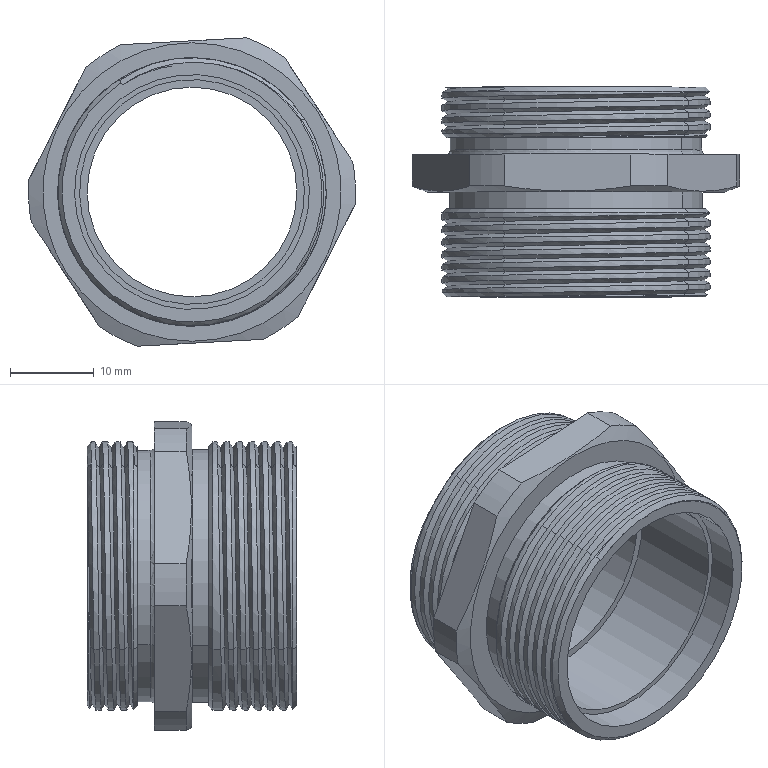Part | SolidWorks | features BaseBody 1 | 1 solid | 158 faces | box 39 x 25 x 36.772 mm | volume 7027 mm3 | spline 84 | cylinder 40 | plane 18 | cone 12 | torus 4 | commonest cylinder face diameters 32 x24 39 x6 25 x2 26.8 x2 28 x2 30 x2